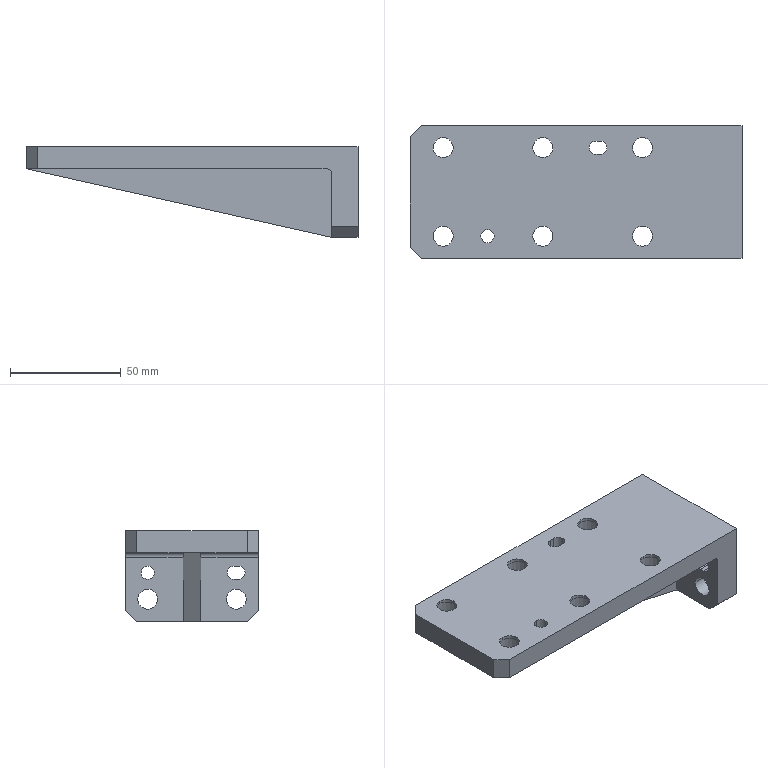Part | 1 solid | 66 faces | box 150 x 60 x 41 mm | volume 116239 mm3 | cylinder 39 | plane 27 | commonest cylinder face diameters 9 x16 15 x12 6 x9 4 x2